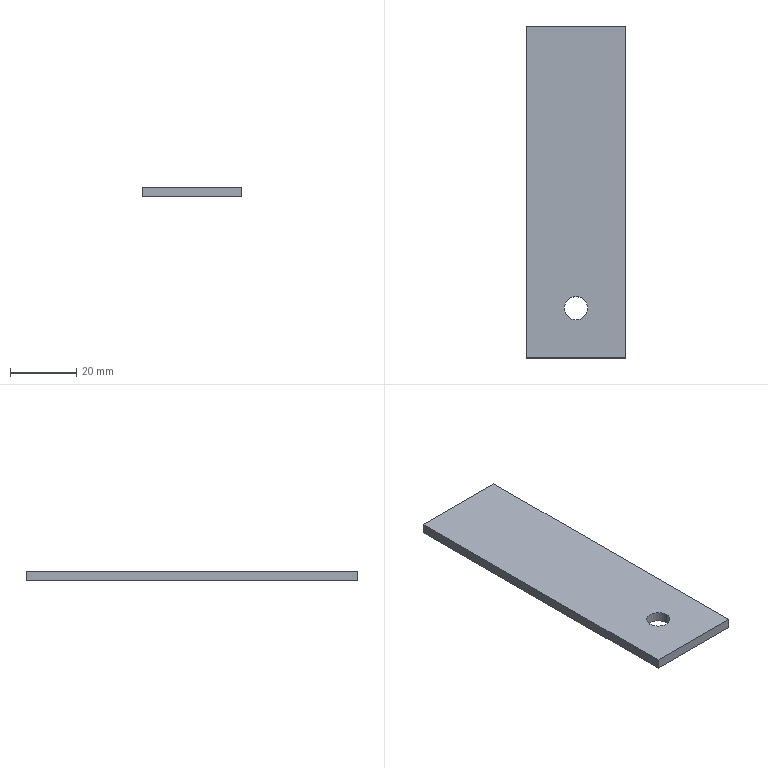Part | STEP file | Microwave Drying Flat Conveyor-CN2500x400-104-102 | 1 solid | 8 faces | box 30 x 100 x 3 mm | volume 8885 mm3 | plane 6 | cylinder 2 | commonest cylinder face diameters 7 x2
STEP:
#1=CARTESIAN_POINT('',(-3.5,-35.,3.));
#2=VERTEX_POINT('',#1);
#3=CARTESIAN_POINT('',(3.5,-35.,3.));
#4=VERTEX_POINT('',#3);
#5=CARTESIAN_POINT('',(0.,-35.,3.));
#6=DIRECTION('',(0.,0.,1.));
#7=DIRECTION('',(1.,0.,0.));
#8=AXIS2_PLACEMENT_3D('',#5,#6,#7);
#9=CIRCLE('',#8,3.5);
#10=EDGE_CURVE('',#2,#4,#9,.T.);
#11=ORIENTED_EDGE('',*,*,#10,.T.);
#12=CARTESIAN_POINT('',(3.5,-35.,0.));
#13=VERTEX_POINT('',#12);
#14=CARTESIAN_POINT('',(3.5,-35.,3.));
#15=DIRECTION('',(0.,0.,-1.));
#16=VECTOR('',#15,1000.);
#17=LINE('',#14,#16);
#18=EDGE_CURVE('',#4,#13,#17,.T.);
#19=ORIENTED_EDGE('',*,*,#18,.T.);
#20=CARTESIAN_POINT('',(-3.5,-35.,0.));
#21=VERTEX_POINT('',#20);
#22=CARTESIAN_POINT('',(0.,-35.,0.));
#23=DIRECTION('',(0.,0.,1.));
#24=DIRECTION('',(1.,0.,0.));
#25=AXIS2_PLACEMENT_3D('',#22,#23,#24);
#26=CIRCLE('',#25,3.5);
#27=EDGE_CURVE('',#21,#13,#26,.T.);
#28=ORIENTED_EDGE('',*,*,#27,.F.);
#29=CARTESIAN_POINT('',(-3.5,-35.,3.));
#30=DIRECTION('',(0.,0.,-1.));
#31=VECTOR('',#30,1000.);
#32=LINE('',#29,#31);
#33=EDGE_CURVE('',#2,#21,#32,.T.);
#34=ORIENTED_EDGE('',*,*,#33,.F.);
#35=EDGE_LOOP('',(#11,#19,#28,#34));
#36=FACE_OUTER_BOUND('',#35,.T.);
#37=CARTESIAN_POINT('',(0.,-35.,3.));
#38=DIRECTION('',(0.,0.,-1.));
#39=DIRECTION('',(-1.,0.,0.));
#40=AXIS2_PLACEMENT_3D('',#37,#38,#39);
#41=CYLINDRICAL_SURFACE('',#40,3.5);
#42=ADVANCED_FACE('',(#36),#41,.F.);
#43=CARTESIAN_POINT('',(15.,-50.,3.));
#44=VERTEX_POINT('',#43);
#45=CARTESIAN_POINT('',(15.,50.,3.));
#46=VERTEX_POINT('',#45);
#47=CARTESIAN_POINT('',(15.,50.,3.));
#48=DIRECTION('',(0.,1.,0.));
#49=VECTOR('',#48,1000.);
#50=LINE('',#47,#49);
#51=EDGE_CURVE('',#44,#46,#50,.T.);
#52=ORIENTED_EDGE('',*,*,#51,.T.);
#53=CARTESIAN_POINT('',(-15.,50.,3.));
#54=VERTEX_POINT('',#53);
#55=CARTESIAN_POINT('',(-15.,50.,3.));
#56=DIRECTION('',(-1.,0.,0.));
#57=VECTOR('',#56,1000.);
#58=LINE('',#55,#57);
#59=EDGE_CURVE('',#46,#54,#58,.T.);
#60=ORIENTED_EDGE('',*,*,#59,.T.);
#61=CARTESIAN_POINT('',(-15.,-50.,3.));
#62=VERTEX_POINT('',#61);
#63=CARTESIAN_POINT('',(-15.,50.,3.));
#64=DIRECTION('',(0.,-1.,0.));
#65=VECTOR('',#64,1000.);
#66=LINE('',#63,#65);
#67=EDGE_CURVE('',#54,#62,#66,.T.);
#68=ORIENTED_EDGE('',*,*,#67,.T.);
#69=CARTESIAN_POINT('',(-15.,-50.,3.));
#70=DIRECTION('',(1.,0.,0.));
#71=VECTOR('',#70,1000.);
#72=LINE('',#69,#71);
#73=EDGE_CURVE('',#62,#44,#72,.T.);
#74=ORIENTED_EDGE('',*,*,#73,.T.);
#75=EDGE_LOOP('',(#52,#60,#68,#74));
#76=FACE_OUTER_BOUND('',#75,.T.);
#77=ORIENTED_EDGE('',*,*,#10,.F.);
#78=CARTESIAN_POINT('',(0.,-35.,3.));
#79=DIRECTION('',(0.,0.,1.));
#80=DIRECTION('',(1.,0.,0.));
#81=AXIS2_PLACEMENT_3D('',#78,#79,#80);
#82=CIRCLE('',#81,3.5);
#83=EDGE_CURVE('',#4,#2,#82,.T.);
#84=ORIENTED_EDGE('',*,*,#83,.F.);
#85=EDGE_LOOP('',(#77,#84));
#86=FACE_BOUND('',#85,.T.);
#87=CARTESIAN_POINT('',(0.,0.,3.));
#88=DIRECTION('',(0.,0.,1.));
#89=DIRECTION('',(1.,0.,0.));
#90=AXIS2_PLACEMENT_3D('',#87,#88,#89);
#91=PLANE('',#90);
#92=ADVANCED_FACE('',(#76,#86),#91,.T.);
#93=CARTESIAN_POINT('',(15.,-50.,0.));
#94=VERTEX_POINT('',#93);
#95=CARTESIAN_POINT('',(15.,50.,0.));
#96=VERTEX_POINT('',#95);
#97=CARTESIAN_POINT('',(15.,50.,0.));
#98=DIRECTION('',(0.,1.,0.));
#99=VECTOR('',#98,1000.);
#100=LINE('',#97,#99);
#101=EDGE_CURVE('',#94,#96,#100,.T.);
#102=ORIENTED_EDGE('',*,*,#101,.F.);
#103=CARTESIAN_POINT('',(-15.,-50.,0.));
#104=VERTEX_POINT('',#103);
#105=CARTESIAN_POINT('',(-15.,-50.,0.));
#106=DIRECTION('',(1.,0.,0.));
#107=VECTOR('',#106,1000.);
#108=LINE('',#105,#107);
#109=EDGE_CURVE('',#104,#94,#108,.T.);
#110=ORIENTED_EDGE('',*,*,#109,.F.);
#111=CARTESIAN_POINT('',(-15.,50.,0.));
#112=VERTEX_POINT('',#111);
#113=CARTESIAN_POINT('',(-15.,50.,0.));
#114=DIRECTION('',(0.,-1.,0.));
#115=VECTOR('',#114,1000.);
#116=LINE('',#113,#115);
#117=EDGE_CURVE('',#112,#104,#116,.T.);
#118=ORIENTED_EDGE('',*,*,#117,.F.);
#119=CARTESIAN_POINT('',(-15.,50.,0.));
#120=DIRECTION('',(-1.,0.,0.));
#121=VECTOR('',#120,1000.);
#122=LINE('',#119,#121);
#123=EDGE_CURVE('',#96,#112,#122,.T.);
#124=ORIENTED_EDGE('',*,*,#123,.F.);
#125=EDGE_LOOP('',(#102,#110,#118,#124));
#126=FACE_OUTER_BOUND('',#125,.T.);
#127=ORIENTED_EDGE('',*,*,#27,.T.);
#128=CARTESIAN_POINT('',(0.,-35.,0.));
#129=DIRECTION('',(0.,0.,1.));
#130=DIRECTION('',(1.,0.,0.));
#131=AXIS2_PLACEMENT_3D('',#128,#129,#130);
#132=CIRCLE('',#131,3.5);
#133=EDGE_CURVE('',#13,#21,#132,.T.);
#134=ORIENTED_EDGE('',*,*,#133,.T.);
#135=EDGE_LOOP('',(#127,#134));
#136=FACE_BOUND('',#135,.T.);
#137=CARTESIAN_POINT('',(0.,0.,0.));
#138=DIRECTION('',(0.,0.,1.));
#139=DIRECTION('',(1.,0.,0.));
#140=AXIS2_PLACEMENT_3D('',#137,#138,#139);
#141=PLANE('',#140);
#142=ADVANCED_FACE('',(#126,#136),#141,.F.);
#143=ORIENTED_EDGE('',*,*,#101,.T.);
#144=CARTESIAN_POINT('',(15.,50.,3.));
#145=DIRECTION('',(0.,0.,-1.));
#146=VECTOR('',#145,1000.);
#147=LINE('',#144,#146);
#148=EDGE_CURVE('',#46,#96,#147,.T.);
#149=ORIENTED_EDGE('',*,*,#148,.F.);
#150=ORIENTED_EDGE('',*,*,#51,.F.);
#151=CARTESIAN_POINT('',(15.,-50.,3.));
#152=DIRECTION('',(0.,0.,-1.));
#153=VECTOR('',#152,1000.);
#154=LINE('',#151,#153);
#155=EDGE_CURVE('',#44,#94,#154,.T.);
#156=ORIENTED_EDGE('',*,*,#155,.T.);
#157=EDGE_LOOP('',(#143,#149,#150,#156));
#158=FACE_OUTER_BOUND('',#157,.T.);
#159=CARTESIAN_POINT('',(15.,50.,3.));
#160=DIRECTION('',(-1.,0.,0.));
#161=DIRECTION('',(0.,-1.,0.));
#162=AXIS2_PLACEMENT_3D('',#159,#160,#161);
#163=PLANE('',#162);
#164=ADVANCED_FACE('',(#158),#163,.F.);
#165=ORIENTED_EDGE('',*,*,#123,.T.);
#166=CARTESIAN_POINT('',(-15.,50.,3.));
#167=DIRECTION('',(0.,0.,-1.));
#168=VECTOR('',#167,1000.);
#169=LINE('',#166,#168);
#170=EDGE_CURVE('',#54,#112,#169,.T.);
#171=ORIENTED_EDGE('',*,*,#170,.F.);
#172=ORIENTED_EDGE('',*,*,#59,.F.);
#173=ORIENTED_EDGE('',*,*,#148,.T.);
#174=EDGE_LOOP('',(#165,#171,#172,#173));
#175=FACE_OUTER_BOUND('',#174,.T.);
#176=CARTESIAN_POINT('',(-15.,50.,3.));
#177=DIRECTION('',(0.,-1.,0.));
#178=DIRECTION('',(0.,0.,-1.));
#179=AXIS2_PLACEMENT_3D('',#176,#177,#178);
#180=PLANE('',#179);
#181=ADVANCED_FACE('',(#175),#180,.F.);
#182=ORIENTED_EDGE('',*,*,#117,.T.);
#183=CARTESIAN_POINT('',(-15.,-50.,3.));
#184=DIRECTION('',(0.,0.,-1.));
#185=VECTOR('',#184,1000.);
#186=LINE('',#183,#185);
#187=EDGE_CURVE('',#62,#104,#186,.T.);
#188=ORIENTED_EDGE('',*,*,#187,.F.);
#189=ORIENTED_EDGE('',*,*,#67,.F.);
#190=ORIENTED_EDGE('',*,*,#170,.T.);
#191=EDGE_LOOP('',(#182,#188,#189,#190));
#192=FACE_OUTER_BOUND('',#191,.T.);
#193=CARTESIAN_POINT('',(-15.,50.,3.));
#194=DIRECTION('',(1.,0.,0.));
#195=DIRECTION('',(0.,1.,0.));
#196=AXIS2_PLACEMENT_3D('',#193,#194,#195);
#197=PLANE('',#196);
#198=ADVANCED_FACE('',(#192),#197,.F.);
#199=ORIENTED_EDGE('',*,*,#109,.T.);
#200=ORIENTED_EDGE('',*,*,#155,.F.);
#201=ORIENTED_EDGE('',*,*,#73,.F.);
#202=ORIENTED_EDGE('',*,*,#187,.T.);
#203=EDGE_LOOP('',(#199,#200,#201,#202));
#204=FACE_OUTER_BOUND('',#203,.T.);
#205=CARTESIAN_POINT('',(-15.,-50.,3.));
#206=DIRECTION('',(0.,1.,0.));
#207=DIRECTION('',(0.,0.,1.));
#208=AXIS2_PLACEMENT_3D('',#205,#206,#207);
#209=PLANE('',#208);
#210=ADVANCED_FACE('',(#204),#209,.F.);
#211=ORIENTED_EDGE('',*,*,#18,.F.);
#212=ORIENTED_EDGE('',*,*,#83,.T.);
#213=ORIENTED_EDGE('',*,*,#33,.T.);
#214=ORIENTED_EDGE('',*,*,#133,.F.);
#215=EDGE_LOOP('',(#211,#212,#213,#214));
#216=FACE_OUTER_BOUND('',#215,.T.);
#217=CARTESIAN_POINT('',(0.,-35.,3.));
#218=DIRECTION('',(0.,0.,-1.));
#219=DIRECTION('',(-1.,0.,0.));
#220=AXIS2_PLACEMENT_3D('',#217,#218,#219);
#221=CYLINDRICAL_SURFACE('',#220,3.5);
#222=ADVANCED_FACE('',(#216),#221,.F.);
#223=CLOSED_SHELL('',(#42,#92,#142,#164,#181,#198,#210,#222));
#224=MANIFOLD_SOLID_BREP('',#223);
#225=CARTESIAN_POINT('',(0.,0.,0.));
#226=DIRECTION('',(0.,0.,1.));
#227=DIRECTION('',(1.,0.,0.));
#228=AXIS2_PLACEMENT_3D('',#225,#226,#227);
#229=(LENGTH_UNIT()NAMED_UNIT(*)SI_UNIT(.MILLI.,.METRE.));
#230=UNCERTAINTY_MEASURE_WITH_UNIT(LENGTH_MEASURE(0.00001),#229,'','');
#231=(NAMED_UNIT(*)PLANE_ANGLE_UNIT()SI_UNIT($,.RADIAN.));
#232=(NAMED_UNIT(*)SI_UNIT($,.STERADIAN.)SOLID_ANGLE_UNIT());
#233=(GEOMETRIC_REPRESENTATION_CONTEXT(3)GLOBAL_UNCERTAINTY_ASSIGNED_CONTEXT((#230))GLOBAL_UNIT_ASSIGNED_CONTEXT((#229,#231,#232))REPRESENTATION_CONTEXT('',''));
#234=ADVANCED_BREP_SHAPE_REPRESENTATION('',(#224,#228),#233);